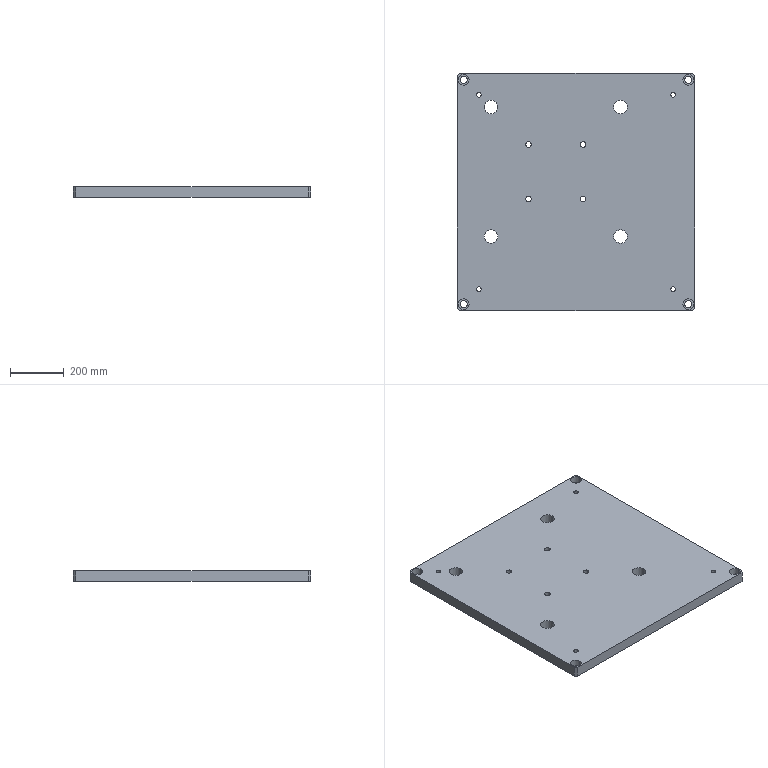Part | SolidWorks | features Extrusion 1, ICE 1 | 1 solid | 54 faces | box 880 x 880 x 40 mm | volume 30404621 mm3 | cylinder 40 | plane 14 | commonest cylinder face diameters 17.294 x8 20.752 x8 26 x8 40 x8 50 x8